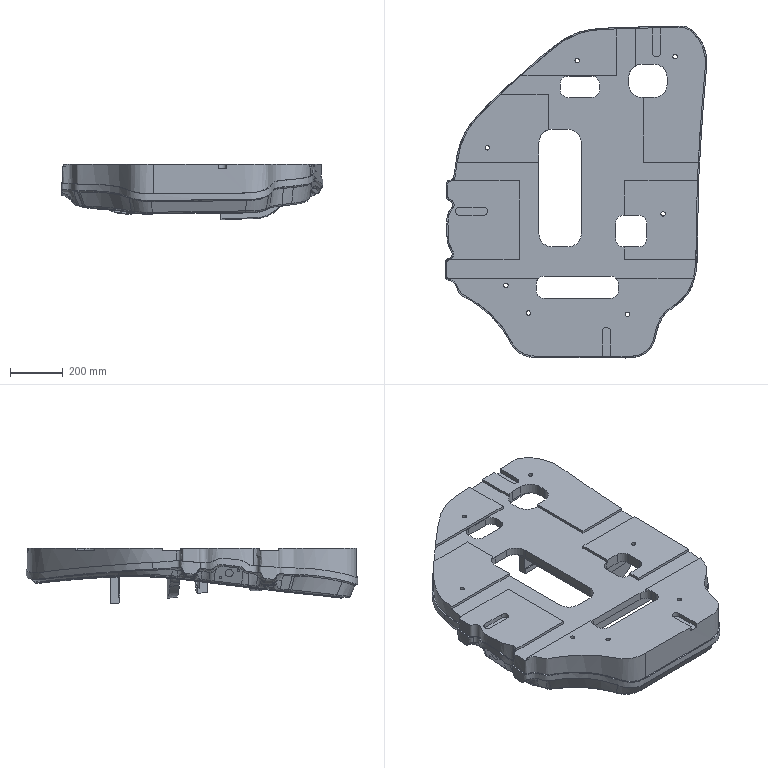Part | NX | features solid 2 | 1 solid | 549 faces | box 990.642 x 1256 x 209.924 mm | volume 66341821 mm3 | spline 335 | plane 152 | cylinder 58 | cone 4 | commonest cylinder face diameters 60 x16 25 x13 32 x8 100 x8 17 x7 16 x4